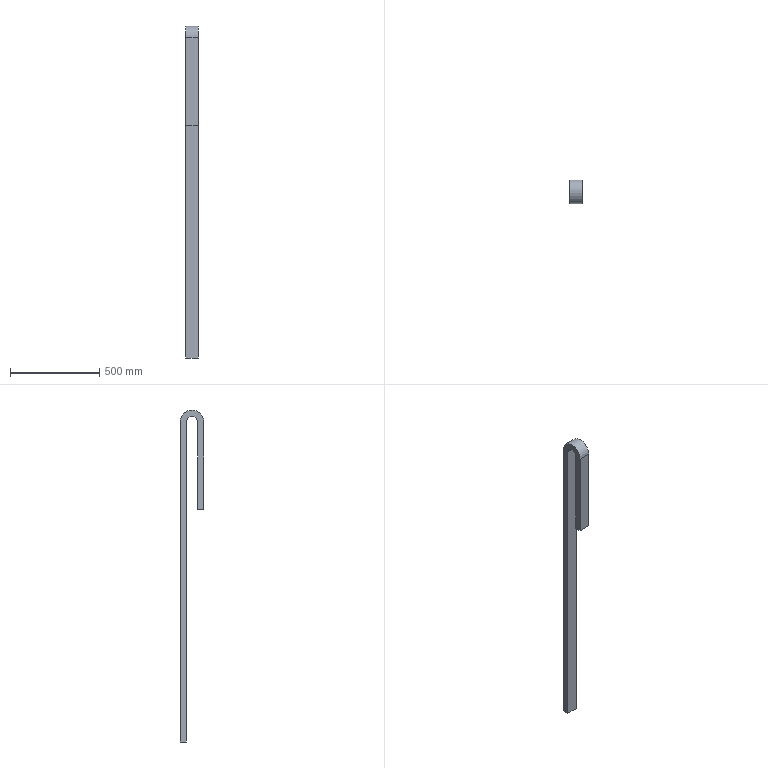Part | SolidWorks | features ExtruThin 1 | 1 solid | 10 faces | box 68 x 132.441 x 1862 mm | volume 5807055 mm3 | plane 8 | cylinder 2 | commonest cylinder face diameters 62.441 x1 132.441 x1
STEP:
#1=CARTESIAN_POINT('',(-52.992,-141.23,559.622));
#2=VERTEX_POINT('',#1);
#3=CARTESIAN_POINT('',(-52.992,-141.23,-1235.693));
#4=VERTEX_POINT('',#3);
#5=CARTESIAN_POINT('',(-52.992,-141.23,-1235.693));
#6=DIRECTION('',(0.,0.,-1.));
#7=VECTOR('',#6,1000.);
#8=LINE('',#5,#7);
#9=EDGE_CURVE('',#2,#4,#8,.T.);
#10=ORIENTED_EDGE('',*,*,#9,.T.);
#11=CARTESIAN_POINT('',(-120.992,-141.23,-1235.693));
#12=VERTEX_POINT('',#11);
#13=CARTESIAN_POINT('',(-120.992,-141.23,-1235.693));
#14=DIRECTION('',(1.,0.,0.));
#15=VECTOR('',#14,1000.);
#16=LINE('',#13,#15);
#17=EDGE_CURVE('',#12,#4,#16,.T.);
#18=ORIENTED_EDGE('',*,*,#17,.F.);
#19=CARTESIAN_POINT('',(-120.992,-141.23,559.622));
#20=VERTEX_POINT('',#19);
#21=CARTESIAN_POINT('',(-120.992,-141.23,-1235.693));
#22=DIRECTION('',(0.,0.,-1.));
#23=VECTOR('',#22,1000.);
#24=LINE('',#21,#23);
#25=EDGE_CURVE('',#20,#12,#24,.T.);
#26=ORIENTED_EDGE('',*,*,#25,.F.);
#27=CARTESIAN_POINT('',(-120.992,-141.23,559.622));
#28=DIRECTION('',(1.,0.,0.));
#29=VECTOR('',#28,1000.);
#30=LINE('',#27,#29);
#31=EDGE_CURVE('',#20,#2,#30,.T.);
#32=ORIENTED_EDGE('',*,*,#31,.T.);
#33=EDGE_LOOP('',(#10,#18,#26,#32));
#34=FACE_OUTER_BOUND('',#33,.T.);
#35=CARTESIAN_POINT('',(-120.992,-141.23,-1235.693));
#36=DIRECTION('',(0.,-1.,0.));
#37=DIRECTION('',(1.,0.,0.));
#38=AXIS2_PLACEMENT_3D('',#35,#36,#37);
#39=PLANE('',#38);
#40=ADVANCED_FACE('',(#34),#39,.F.);
#41=CARTESIAN_POINT('',(-52.992,-176.23,-1235.693));
#42=VERTEX_POINT('',#41);
#43=CARTESIAN_POINT('',(-52.992,-176.23,-1235.693));
#44=DIRECTION('',(0.,1.,0.));
#45=VECTOR('',#44,1000.);
#46=LINE('',#43,#45);
#47=EDGE_CURVE('',#42,#4,#46,.T.);
#48=ORIENTED_EDGE('',*,*,#47,.F.);
#49=CARTESIAN_POINT('',(-120.992,-176.23,-1235.693));
#50=VERTEX_POINT('',#49);
#51=CARTESIAN_POINT('',(-120.992,-176.23,-1235.693));
#52=DIRECTION('',(1.,0.,0.));
#53=VECTOR('',#52,1000.);
#54=LINE('',#51,#53);
#55=EDGE_CURVE('',#50,#42,#54,.T.);
#56=ORIENTED_EDGE('',*,*,#55,.F.);
#57=CARTESIAN_POINT('',(-120.992,-176.23,-1235.693));
#58=DIRECTION('',(0.,1.,0.));
#59=VECTOR('',#58,1000.);
#60=LINE('',#57,#59);
#61=EDGE_CURVE('',#50,#12,#60,.T.);
#62=ORIENTED_EDGE('',*,*,#61,.T.);
#63=ORIENTED_EDGE('',*,*,#17,.T.);
#64=EDGE_LOOP('',(#48,#56,#62,#63));
#65=FACE_OUTER_BOUND('',#64,.T.);
#66=CARTESIAN_POINT('',(-120.992,-176.23,-1235.693));
#67=DIRECTION('',(0.,0.,-1.));
#68=DIRECTION('',(-1.,0.,0.));
#69=AXIS2_PLACEMENT_3D('',#66,#67,#68);
#70=PLANE('',#69);
#71=ADVANCED_FACE('',(#65),#70,.T.);
#72=CARTESIAN_POINT('',(-52.992,-176.23,559.622));
#73=VERTEX_POINT('',#72);
#74=CARTESIAN_POINT('',(-52.992,-176.23,-1235.693));
#75=DIRECTION('',(0.,0.,-1.));
#76=VECTOR('',#75,1000.);
#77=LINE('',#74,#76);
#78=EDGE_CURVE('',#73,#42,#77,.T.);
#79=ORIENTED_EDGE('',*,*,#78,.F.);
#80=CARTESIAN_POINT('',(-120.992,-176.23,559.622));
#81=VERTEX_POINT('',#80);
#82=CARTESIAN_POINT('',(-120.992,-176.23,559.622));
#83=DIRECTION('',(1.,0.,0.));
#84=VECTOR('',#83,1000.);
#85=LINE('',#82,#84);
#86=EDGE_CURVE('',#81,#73,#85,.T.);
#87=ORIENTED_EDGE('',*,*,#86,.F.);
#88=CARTESIAN_POINT('',(-120.992,-176.23,-1235.693));
#89=DIRECTION('',(0.,0.,-1.));
#90=VECTOR('',#89,1000.);
#91=LINE('',#88,#90);
#92=EDGE_CURVE('',#81,#50,#91,.T.);
#93=ORIENTED_EDGE('',*,*,#92,.T.);
#94=ORIENTED_EDGE('',*,*,#55,.T.);
#95=EDGE_LOOP('',(#79,#87,#93,#94));
#96=FACE_OUTER_BOUND('',#95,.T.);
#97=CARTESIAN_POINT('',(-120.992,-176.23,-1235.693));
#98=DIRECTION('',(0.,-1.,0.));
#99=DIRECTION('',(1.,0.,0.));
#100=AXIS2_PLACEMENT_3D('',#97,#98,#99);
#101=PLANE('',#100);
#102=ADVANCED_FACE('',(#96),#101,.T.);
#103=CARTESIAN_POINT('',(-52.992,-238.671,559.622));
#104=VERTEX_POINT('',#103);
#105=CARTESIAN_POINT('',(-52.992,-207.45,559.622));
#106=DIRECTION('',(-1.,0.,0.));
#107=DIRECTION('',(0.,0.,-1.));
#108=AXIS2_PLACEMENT_3D('',#105,#106,#107);
#109=CIRCLE('',#108,31.22);
#110=EDGE_CURVE('',#104,#73,#109,.T.);
#111=ORIENTED_EDGE('',*,*,#110,.F.);
#112=CARTESIAN_POINT('',(-120.992,-238.671,559.622));
#113=VERTEX_POINT('',#112);
#114=CARTESIAN_POINT('',(-120.992,-238.671,559.622));
#115=DIRECTION('',(1.,0.,0.));
#116=VECTOR('',#115,1000.);
#117=LINE('',#114,#116);
#118=EDGE_CURVE('',#113,#104,#117,.T.);
#119=ORIENTED_EDGE('',*,*,#118,.F.);
#120=CARTESIAN_POINT('',(-120.992,-207.45,559.622));
#121=DIRECTION('',(-1.,0.,0.));
#122=DIRECTION('',(0.,0.,-1.));
#123=AXIS2_PLACEMENT_3D('',#120,#121,#122);
#124=CIRCLE('',#123,31.22);
#125=EDGE_CURVE('',#113,#81,#124,.T.);
#126=ORIENTED_EDGE('',*,*,#125,.T.);
#127=ORIENTED_EDGE('',*,*,#86,.T.);
#128=EDGE_LOOP('',(#111,#119,#126,#127));
#129=FACE_OUTER_BOUND('',#128,.T.);
#130=CARTESIAN_POINT('',(-120.992,-207.45,559.622));
#131=DIRECTION('',(1.,0.,0.));
#132=DIRECTION('',(0.,1.,0.));
#133=AXIS2_PLACEMENT_3D('',#130,#131,#132);
#134=CYLINDRICAL_SURFACE('',#133,31.22);
#135=ADVANCED_FACE('',(#129),#134,.F.);
#136=CARTESIAN_POINT('',(-52.992,-238.671,68.058));
#137=VERTEX_POINT('',#136);
#138=CARTESIAN_POINT('',(-52.992,-238.671,68.058));
#139=DIRECTION('',(0.,0.,1.));
#140=VECTOR('',#139,1000.);
#141=LINE('',#138,#140);
#142=EDGE_CURVE('',#137,#104,#141,.T.);
#143=ORIENTED_EDGE('',*,*,#142,.F.);
#144=CARTESIAN_POINT('',(-120.992,-238.671,68.058));
#145=VERTEX_POINT('',#144);
#146=CARTESIAN_POINT('',(-120.992,-238.671,68.058));
#147=DIRECTION('',(1.,0.,0.));
#148=VECTOR('',#147,1000.);
#149=LINE('',#146,#148);
#150=EDGE_CURVE('',#145,#137,#149,.T.);
#151=ORIENTED_EDGE('',*,*,#150,.F.);
#152=CARTESIAN_POINT('',(-120.992,-238.671,68.058));
#153=DIRECTION('',(0.,0.,1.));
#154=VECTOR('',#153,1000.);
#155=LINE('',#152,#154);
#156=EDGE_CURVE('',#145,#113,#155,.T.);
#157=ORIENTED_EDGE('',*,*,#156,.T.);
#158=ORIENTED_EDGE('',*,*,#118,.T.);
#159=EDGE_LOOP('',(#143,#151,#157,#158));
#160=FACE_OUTER_BOUND('',#159,.T.);
#161=CARTESIAN_POINT('',(-120.992,-238.671,68.058));
#162=DIRECTION('',(0.,1.,0.));
#163=DIRECTION('',(-1.,0.,0.));
#164=AXIS2_PLACEMENT_3D('',#161,#162,#163);
#165=PLANE('',#164);
#166=ADVANCED_FACE('',(#160),#165,.T.);
#167=CARTESIAN_POINT('',(-52.992,-273.671,68.058));
#168=VERTEX_POINT('',#167);
#169=CARTESIAN_POINT('',(-52.992,-273.671,68.058));
#170=DIRECTION('',(0.,1.,0.));
#171=VECTOR('',#170,1000.);
#172=LINE('',#169,#171);
#173=EDGE_CURVE('',#168,#137,#172,.T.);
#174=ORIENTED_EDGE('',*,*,#173,.F.);
#175=CARTESIAN_POINT('',(-120.992,-273.671,68.058));
#176=VERTEX_POINT('',#175);
#177=CARTESIAN_POINT('',(-120.992,-273.671,68.058));
#178=DIRECTION('',(1.,0.,0.));
#179=VECTOR('',#178,1000.);
#180=LINE('',#177,#179);
#181=EDGE_CURVE('',#176,#168,#180,.T.);
#182=ORIENTED_EDGE('',*,*,#181,.F.);
#183=CARTESIAN_POINT('',(-120.992,-273.671,68.058));
#184=DIRECTION('',(0.,1.,0.));
#185=VECTOR('',#184,1000.);
#186=LINE('',#183,#185);
#187=EDGE_CURVE('',#176,#145,#186,.T.);
#188=ORIENTED_EDGE('',*,*,#187,.T.);
#189=ORIENTED_EDGE('',*,*,#150,.T.);
#190=EDGE_LOOP('',(#174,#182,#188,#189));
#191=FACE_OUTER_BOUND('',#190,.T.);
#192=CARTESIAN_POINT('',(-120.992,-273.671,68.058));
#193=DIRECTION('',(0.,0.,-1.));
#194=DIRECTION('',(-1.,0.,0.));
#195=AXIS2_PLACEMENT_3D('',#192,#193,#194);
#196=PLANE('',#195);
#197=ADVANCED_FACE('',(#191),#196,.T.);
#198=CARTESIAN_POINT('',(-52.992,-273.671,559.622));
#199=VERTEX_POINT('',#198);
#200=CARTESIAN_POINT('',(-52.992,-273.671,68.058));
#201=DIRECTION('',(0.,0.,1.));
#202=VECTOR('',#201,1000.);
#203=LINE('',#200,#202);
#204=EDGE_CURVE('',#168,#199,#203,.T.);
#205=ORIENTED_EDGE('',*,*,#204,.T.);
#206=CARTESIAN_POINT('',(-120.992,-273.671,559.622));
#207=VERTEX_POINT('',#206);
#208=CARTESIAN_POINT('',(-120.992,-273.671,559.622));
#209=DIRECTION('',(1.,0.,0.));
#210=VECTOR('',#209,1000.);
#211=LINE('',#208,#210);
#212=EDGE_CURVE('',#207,#199,#211,.T.);
#213=ORIENTED_EDGE('',*,*,#212,.F.);
#214=CARTESIAN_POINT('',(-120.992,-273.671,68.058));
#215=DIRECTION('',(0.,0.,1.));
#216=VECTOR('',#215,1000.);
#217=LINE('',#214,#216);
#218=EDGE_CURVE('',#176,#207,#217,.T.);
#219=ORIENTED_EDGE('',*,*,#218,.F.);
#220=ORIENTED_EDGE('',*,*,#181,.T.);
#221=EDGE_LOOP('',(#205,#213,#219,#220));
#222=FACE_OUTER_BOUND('',#221,.T.);
#223=CARTESIAN_POINT('',(-120.992,-273.671,68.058));
#224=DIRECTION('',(0.,1.,0.));
#225=DIRECTION('',(-1.,0.,0.));
#226=AXIS2_PLACEMENT_3D('',#223,#224,#225);
#227=PLANE('',#226);
#228=ADVANCED_FACE('',(#222),#227,.F.);
#229=CARTESIAN_POINT('',(-52.992,-207.45,559.622));
#230=DIRECTION('',(-1.,0.,0.));
#231=DIRECTION('',(0.,-1.,0.));
#232=AXIS2_PLACEMENT_3D('',#229,#230,#231);
#233=CIRCLE('',#232,66.22);
#234=EDGE_CURVE('',#199,#2,#233,.T.);
#235=ORIENTED_EDGE('',*,*,#234,.T.);
#236=ORIENTED_EDGE('',*,*,#31,.F.);
#237=CARTESIAN_POINT('',(-120.992,-207.45,559.622));
#238=DIRECTION('',(-1.,0.,0.));
#239=DIRECTION('',(0.,-1.,0.));
#240=AXIS2_PLACEMENT_3D('',#237,#238,#239);
#241=CIRCLE('',#240,66.22);
#242=EDGE_CURVE('',#207,#20,#241,.T.);
#243=ORIENTED_EDGE('',*,*,#242,.F.);
#244=ORIENTED_EDGE('',*,*,#212,.T.);
#245=EDGE_LOOP('',(#235,#236,#243,#244));
#246=FACE_OUTER_BOUND('',#245,.T.);
#247=CARTESIAN_POINT('',(-120.992,-207.45,559.622));
#248=DIRECTION('',(1.,0.,0.));
#249=DIRECTION('',(0.,1.,0.));
#250=AXIS2_PLACEMENT_3D('',#247,#248,#249);
#251=CYLINDRICAL_SURFACE('',#250,66.22);
#252=ADVANCED_FACE('',(#246),#251,.T.);
#253=ORIENTED_EDGE('',*,*,#25,.T.);
#254=ORIENTED_EDGE('',*,*,#61,.F.);
#255=ORIENTED_EDGE('',*,*,#92,.F.);
#256=ORIENTED_EDGE('',*,*,#125,.F.);
#257=ORIENTED_EDGE('',*,*,#156,.F.);
#258=ORIENTED_EDGE('',*,*,#187,.F.);
#259=ORIENTED_EDGE('',*,*,#218,.T.);
#260=ORIENTED_EDGE('',*,*,#242,.T.);
#261=EDGE_LOOP('',(#253,#254,#255,#256,#257,#258,#259,#260));
#262=FACE_OUTER_BOUND('',#261,.T.);
#263=CARTESIAN_POINT('',(-120.992,-207.45,559.622));
#264=DIRECTION('',(-1.,0.,0.));
#265=DIRECTION('',(0.,0.,-1.));
#266=AXIS2_PLACEMENT_3D('',#263,#264,#265);
#267=PLANE('',#266);
#268=ADVANCED_FACE('',(#262),#267,.T.);
#269=ORIENTED_EDGE('',*,*,#9,.F.);
#270=ORIENTED_EDGE('',*,*,#234,.F.);
#271=ORIENTED_EDGE('',*,*,#204,.F.);
#272=ORIENTED_EDGE('',*,*,#173,.T.);
#273=ORIENTED_EDGE('',*,*,#142,.T.);
#274=ORIENTED_EDGE('',*,*,#110,.T.);
#275=ORIENTED_EDGE('',*,*,#78,.T.);
#276=ORIENTED_EDGE('',*,*,#47,.T.);
#277=EDGE_LOOP('',(#269,#270,#271,#272,#273,#274,#275,#276));
#278=FACE_OUTER_BOUND('',#277,.T.);
#279=CARTESIAN_POINT('',(-52.992,-207.45,559.622));
#280=DIRECTION('',(-1.,0.,0.));
#281=DIRECTION('',(0.,0.,-1.));
#282=AXIS2_PLACEMENT_3D('',#279,#280,#281);
#283=PLANE('',#282);
#284=ADVANCED_FACE('',(#278),#283,.F.);
#285=CLOSED_SHELL('',(#40,#71,#102,#135,#166,#197,#228,#252,#268,#284));
#286=MANIFOLD_SOLID_BREP('',#285);
#287=CARTESIAN_POINT('',(0.,0.,0.));
#288=DIRECTION('',(0.,0.,1.));
#289=DIRECTION('',(1.,0.,0.));
#290=AXIS2_PLACEMENT_3D('',#287,#288,#289);
#291=(LENGTH_UNIT()NAMED_UNIT(*)SI_UNIT(.MILLI.,.METRE.));
#292=UNCERTAINTY_MEASURE_WITH_UNIT(LENGTH_MEASURE(0.00001),#291,'','');
#293=(NAMED_UNIT(*)PLANE_ANGLE_UNIT()SI_UNIT($,.RADIAN.));
#294=(NAMED_UNIT(*)SI_UNIT($,.STERADIAN.)SOLID_ANGLE_UNIT());
#295=(GEOMETRIC_REPRESENTATION_CONTEXT(3)GLOBAL_UNCERTAINTY_ASSIGNED_CONTEXT((#292))GLOBAL_UNIT_ASSIGNED_CONTEXT((#291,#293,#294))REPRESENTATION_CONTEXT('',''));
#296=ADVANCED_BREP_SHAPE_REPRESENTATION('',(#286,#290),#295);